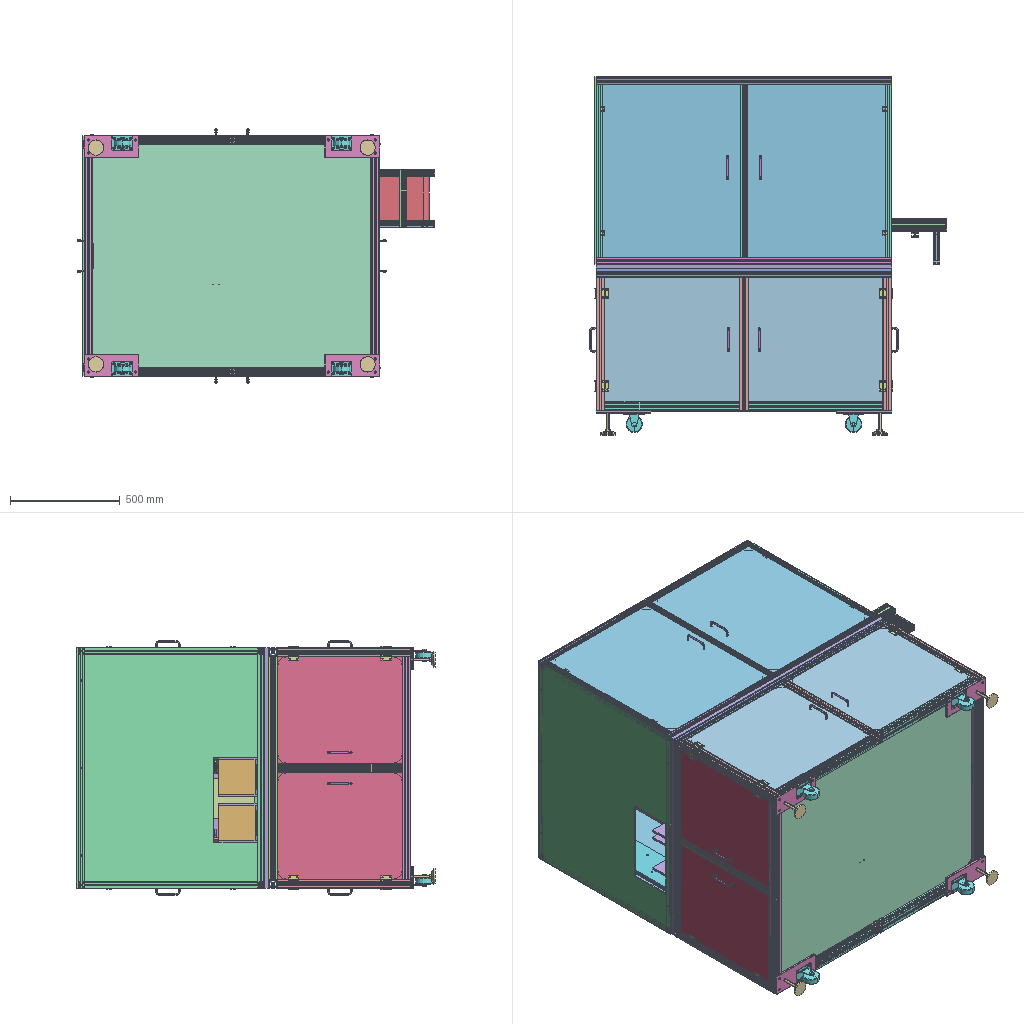Assembly | STEP file | 255 different items | 665 placed | box 1630 x 1635 x 1160 mm
Parts list (item | name | quantity | parent item | size | volume):
1 | 01-01 Bracket post | x6 | in 41 | 40 x 610 x 40 mm | 561060 mm3
2 | 01-03 Bracket crossbar 1 | x2 | in 41 | 40 x 1350 x 40 mm | 1241689 mm3
3 | 01-05 Bracket crossbar 3 | x2 | in 41 | 40 x 1020 x 40 mm | 938165 mm3
4 | 01-06 Bracket crossbar 4 | x2 | in 41 | 40 x 1020 x 40 mm | 938165 mm3
5 | 01-04 Bracket crossbar 2 | x4 | in 41 | 40 x 615 x 40 mm | 565659 mm3
6 | 01-02 Bracket post 2 | x2 | in 41 | 40 x 570 x 40 mm | 524269 mm3
7 | 01-07 Base plate | x1 | in 41 | 20 x 1100 x 1350 mm | 29158066 mm3
8 | 40×40 aluminium angle | x32 | in 41 | 30 x 40 x 40 mm | 8764 mm3
9 | 01-08 Base frame seal plate 1 | x4 | in 41 | 5 x 570 x 490 mm | 144415 mm3
10 | 01-09 Base frame seal plate 2 | x4 | in 41 | 5 x 570 x 615 mm | 180603 mm3
11 | 50 hinge | x16 | in 41 | 47 x 5 x 34 mm | 2311 mm3
12 | Stainless steel handle | x15 | in 41 | 8 x 30 x 112 mm | 7163 mm3
13 | 01-10 Base plate 2 | x1 | in 41 | 10 x 1330 x 1080 mm | 14031243 mm3
14 | 01-13 Coil feed support base plate | x1 | in 41 | 10 x 50 x 50 mm | 22250 mm3
15 | 01-12 Coil feed support plate | x1 | in 41 | 10 x 250 x 50 mm | 123839 mm3
16 | 01-11 Coil feed support shaft | x1 | in 41 | 50 x 40 x 40 mm | 62215 mm3
17 | 01-14 Caster foot cup support plate | x4 | in 41 | 10 x 250 x 100 mm | 245227 mm3
18 | Caster | x4 | in 41 | 70 x 95 x 87.5 mm | 164739 mm3
19 | Foot cup NFJNS16-130 | x4 | in 41 | 70 x 150 x 70 mm | 67181 mm3
20 | 05-01 Turntable | x1 | in 41 | 15 x 500 x 500 mm | 2906258 mm3
21 | 05-02 Turntable shaft | x1 | in 41 | 110 x 258 x 110 mm | 522826 mm3
22 | Bearing 32911 | x2 | in 41 | 80 x 17 x 80 mm | 44892 mm3
23 | 05-03 Turntable seat | x1 | in 41 | 150 x 128 x 150 mm | 603065 mm3
24 | 05-04 Turntable bottom press plate | x1 | in 41 | 10 x 70 x 70 mm | 31647 mm3
25 | 05-05 Fixture | x16 | in 41 | 42 x 40 x 40 mm | 49529 mm3
26 | Magnet dia 10 thickness 6 | x16 | in 41 | 6 x 10 x 10 mm | 467.969 mm3
27 | 05-06 Alignment piece fixing seat | x1 | in 41 | 45 x 45 x 20 mm | 12273 mm3
28 | 05-07 Alignment piece | x1 | in 41 | 2 x 69.821 x 69.821 mm | 5865 mm3
29 | Coupling CPSWWKΦ19-Φ19 (high-rigidity diaphragm type) | x1 | in 41 | 65 x 65 x 77 mm | 150728 mm3
30 | BSHB311 Baishan Motor | x1 | in 41 | 256 x 110 x 110 mm | 2048364 mm3
31 | 05-08 Motor fixing plate | x1 | in 41 | 10 x 160 x 160 mm | 243023 mm3
32 | 05-09 Fixing connection plate 1 | x4 | in 41 | 10 x 149 x 40 mm | 57725 mm3
33 | 05-10 Fixing connection plate 2 | x4 | in 41 | 10 x 149 x 30 mm | 43468 mm3
34 | 06-01 Heat-shrink sleeve shaft | x1 | in 41 | 20.3 x 500 x 20.3 mm | 156269 mm3
35 | Bearing B603ZZ | x4 | in 41 | 5 x 9 x 9 mm | 282.092 mm3
36 | 06-04 Bearing pin | x4 | in 41 | 12 x 3 x 3 mm | 82.729 mm3
37 | 06-02 Support feed wheel | x2 | in 41 | 20 x 25.8 x 25.8 mm | 8769 mm3
38 | 06-05 Support feed wheel shaft | x2 | in 41 | 12 x 12 x 67 mm | 4710 mm3
39 | Bearing B6900ZZ | x2 | in 41 | 6 x 22 x 22 mm | 1808 mm3
40 | circlips for shaft--type a large gb_GB_CONNECTING_PIECE_RING_RRA 10 | x2 | in 41 | 11.5 x 13.997 x 1 mm | 50.603 mm3
41 | 06-06 Driving feed support plate | x1 | in 41 | 10 x 260 x 100 mm | 216439 mm3
42 | 06-07 Bearing cover plate | x2 | in 41 | 2 x 60 x 30 mm | 2906 mm3
43 | hexagon socket head cap screws gb_GB_FASTENER_SCREWS_HSHCS M5X25-N | x4 | in 41 | 30 x 8.5 x 8.5 mm | 732.663 mm3
44 | BS57 Baishan Motor | x4 | in 41 | 98.2 x 56.4 x 56.4 mm | 213692 mm3
45 | 06-08 1-60 gear | x1 | in 41 | 20 x 61.958 x 61.958 mm | 30335 mm3
46 | 06-09 1-40 gear | x2 | in 41 | 20 x 41.938 x 41.938 mm | 14422 mm3
47 | 06-10 Guide mixing wheel support shaft | x4 | in 41 | 8 x 10 x 34 mm | 879.659 mm3
48 | Bearing B685ZZ | x8 | in 41 | 5 x 11 x 11 mm | 376.118 mm3
49 | 06-03 Guide mixing wheel | x4 | in 41 | 30 x 20 x 30 mm | 7202 mm3
50 | 06-11 Driven feed support plate | x1 | in 41 | 10 x 260 x 70 mm | 174356 mm3
51 | 06-12 Driving feed slide plate | x2 | in 41 | 25 x 80 x 70 mm | 132614 mm3
52 | 06-13 Push-pull bearing seat | x2 | in 41 | 16 x 30 x 45 mm | 7960 mm3
53 | Bearing B688ZZ | x2 | in 41 | 5 x 16 x 16 mm | 752.708 mm3
54 | 06-14 Bearing seat cover plate | x2 | in 41 | 5 x 25 x 25 mm | 2010 mm3
55 | 06-15 Slide guide block 1 | x4 | in 41 | 70 x 30 x 25 mm | 33661 mm3
56 | 06-16 M12 screw rod | x2 | in 41 | 12 x 12 x 75 mm | 7389 mm3
57 | Handwheel | x2 | in 41 | 80 x 80 x 65 mm | 48947 mm3
58 | 06-17 Screw locking block | x2 | in 41 | 15 x 60 x 45 mm | 23099 mm3
59 | 06-18 Fixing plate 1 | x1 | in 41 | 15 x 290 x 330 mm | 1410593 mm3
60 | 06-19 Stator fixing plate | x1 | in 41 | 10 x 140 x 140 mm | 144589 mm3
61 | 06-20 Stator core | x1 | in 41 | 81 x 55 x 55 mm | 107790 mm3
62 | 1/8 Φ8 fitting | x1 | in 41 | 28 x 16.166 x 14 mm | 2653 mm3
63 | Inner dia 42.5 wire dia 2.65 O-ring | x4 | in 41 | 47.7 x 47.7 x 2.6 mm | 752.251 mm3
64 | Bearing SB6909ZZ | x2 | in 41 | 12 x 68 x 68 mm | 24454 mm3
65 | 06-21 Rotor | x1 | in 41 | 147.929 x 147.929 x 62 mm | 569803 mm3
66 | 06-22 Stator support plate | x1 | in 41 | 10 x 50 x 50 mm | 13234 mm3
67 | 06-23 Rotor support plate | x1 | in 41 | 10 x 120 x 120 mm | 106201 mm3
68 | 06-25 Cutter slider | x1 | in 41 | 15 x 25 x 31 mm | 8782 mm3
69 | 06-27 Cutter cylinder fixing block | x1 | in 41 | 10 x 30 x 40 mm | 7335 mm3
70 | Cylinder CCOMPANY_AB 10-5_Retract | x1 | in 41 | 15 x 15 x 32.5 mm | 3211 mm3
71 | 06-24 Cutter slide rail | x2 | in 41 | 20 x 10 x 12 mm | 1659 mm3
72 | 06-26 Cutter press block | x1 | in 41 | 15 x 4 x 23 mm | 1168 mm3
73 | Insert blade | x1 | in 41 | 0.5 x 9 x 31.197 mm | 111.216 mm3
74 | 40W JSCC motor | x1 | in 41 | 143 x 125 x 90 mm | 815322 mm3
75 | 06-28 Gear 2-72 | x1 | in 41 | 50 x 147.929 x 147.929 mm | 253016 mm3
76 | 06-29 Up-down adjusting dovetail plate | x1 | in 41 | 230 x 20 x 150 mm | 590829 mm3
77 | 06-31 Dovetail fixing triangle plate | x4 | in 41 | 12 x 59.646 x 59.75 mm | 20836 mm3
78 | 06-32 Up-down adjusting dovetail groove | x1 | in 41 | 260 x 20 x 180 mm | 636123 mm3
79 | 06-30 Up-down dovetail press strip | x1 | in 41 | 260 x 10 x 12.002 mm | 13000 mm3
80 | 06-33 Front-rear adjusting dovetail plate | x1 | in 41 | 160 x 26 x 180 mm | 473686 mm3
81 | 06-34 Front-rear adjusting dovetail groove | x1 | in 41 | 140 x 26 x 110 mm | 222237 mm3
82 | 06-35 Front-rear dovetail press strip | x1 | in 41 | 140 x 16 x 16.203 mm | 11200 mm3
83 | 06-36 Front-rear dovetail base plate | x1 | in 41 | 10 x 140 x 240 mm | 326475 mm3
84 | 06-37 Heat-shrink tube support column | x4 | in 41 | 12 x 400 x 30 mm | 142471 mm3
85 | 06-38 Heat-shrink tube support crossbar | x2 | in 41 | 10 x 30 x 330 mm | 96911 mm3
86 | 06-39 Heat-shrink tube guide shaft | x3 | in 41 | 246 x 20 x 20 mm | 76812 mm3
87 | Inner dia 6 wire dia 1.8 O-ring | x1 | in 41 | 9.6 x 9.6 x 1.8 mm | 62.351 mm3
88 | 06-40 Flat key | x2 | in 41 | 3 x 3 x 13 mm | 111.206 mm3
89 | 40W JSCC gear motor | x1 | in 41 | 78 x 90 x 90 mm | 369652 mm3
90 | 02-04 Side frame | x1 | in 41 | 60 x 1495 x 30 mm | 1200559 mm3
91 | 02-03 Driving mixing drum support seat | x1 | in 41 | 60 x 60 x 30 mm | 91539 mm3
92 | Bearing 6802zz | x6 | in 41 | 5 x 24 x 24 mm | 1309 mm3
93 | 02-01 Driving mixing drum | x1 | in 41 | 50 x 50 x 271 mm | 629819 mm3
94 | 02-05 Driving mixing drum support seat 2 | x1 | in 41 | 60 x 60 x 30 mm | 91539 mm3
95 | 02-06 Side frame 2 | x1 | in 41 | 60 x 1495 x 30 mm | 1313620 mm3
96 | 02-07 25B driving sprocket | x1 | in 41 | 11 x 43.573 x 43.573 mm | 7127 mm3
97 | 02-08 Driving sprocket key | x1 | in 41 | 4 x 4 x 9.5 mm | 137.34 mm3
98 | 02-10 Motor fixing plate | x1 | in 41 | 30 x 130 x 100 mm | 33387 mm3
99 | Motor JSCC 25W | x1 | in 41 | 208 x 115 x 80 mm | 1081551 mm3
100 | 02-09 Motor sprocket | x1 | in 41 | 14 x 43.574 x 43.574 mm | 9063 mm3
101 | 25B chain | x1 | in 41 | 8.6 x 159.55 x 51.6 mm | 26237 mm3
102 | 02-11 Belt line support plate | x1 | in 41 | 1350 x 22 x 204 mm | 495672 mm3
103 | 02-12 Tensioning block 1 | x1 | in 41 | 20 x 32 x 32 mm | 16333 mm3
104 | 02-13 Tensioning block 2 | x1 | in 41 | 20 x 32 x 32 mm | 13018 mm3
105 | 02-02 Driven mixing drum | x1 | in 41 | 50 x 50 x 214 mm | 578580 mm3
106 | 02-14 Adjusting plate | x2 | in 41 | 5 x 60 x 30 mm | 8368 mm3
107 | 02-15 Belt line connecting rod | x4 | in 41 | 30 x 264 x 30 mm | 111601 mm3
108 | 02-15 Conveyor belt | x1 | in 41 | 200 x 54 x 1534 mm | 1249345 mm3
109 | 02-16 Belt line support foot | x8 | in 41 | 30 x 150 x 30 mm | 64799 mm3
110 | TN-16×125-S Extend | x1 | in 41 | 21 x 318 x 54 mm | 212013 mm3
111 | 02-17 Pusher cylinder fixing plate | x1 | in 41 | 10 x 264 x 120 mm | 277247 mm3
112 | Φ8 guide shaft seat | x4 | in 41 | 14 x 32.8 x 42 mm | 8820 mm3
113 | 02-18 Pull-off block | x1 | in 41 | 10 x 14 x 45 mm | 4364 mm3
114 | 02-19 Separating mechanism seal plate | x1 | in 41 | 15 x 350 x 264 mm | 1110870 mm3
115 | 02-20 Φ8 polished rod | x2 | in 41 | 244 x 8 x 8 mm | 12259 mm3
116 | Cylinder TN-16-10-S Retract | x1 | in 41 | 21 x 78 x 54 mm | 81436 mm3
117 | 02-21 Push plate | x1 | in 41 | 15 x 120 x 171.5 mm | 143256 mm3
118 | 02-22 Push connecting block | x1 | in 41 | 15 x 35 x 112 mm | 46704 mm3
119 | Linear bearing LMU8 | x6 | in 41 | 24 x 15 x 15 mm | 2999 mm3
120 | 02-23 Sprocket cover | x1 | in 41 | 40 x 180 x 80 mm | 22772 mm3
121 | 02-24 Battery support plate | x1 | in 41 | 120 x 60 x 120.818 mm | 18521 mm3
122 | Linear bearing LHFRD 16 | x4 | in 41 | 48 x 48 x 56 mm | 29540 mm3
123 | Lead screw head | x3 | in 41 | 44 x 50 x 34 mm | 38804 mm3
124 | 03-01 Loading-unloading side plate 1 | x2 | in 41 | 10 x 210 x 180 mm | 373986 mm3
125 | 03-02 Loading-unloading side plate 2 | x4 | in 41 | 10 x 210 x 168 mm | 351568 mm3
126 | 300 Lead screw | x2 | in 41 | 15 x 15 x 300 mm | 45152 mm3
127 | Bearing SB6800ZZ | x2 | in 41 | 5 x 19 x 19 mm | 1023 mm3
128 | 03-03 Tray support plate | x2 | in 41 | 15 x 168 x 160 mm | 317269 mm3
129 | Coupling CPJC 20 RD φ6.35-φ8 | x2 | in 41 | 30 x 20 x 20 mm | 7655 mm3
130 | 03-04 Bearing cover plate | x2 | in 41 | 5 x 36 x 36 mm | 3710 mm3
131 | 03-05 Motor fixing plate | x2 | in 41 | 8 x 70 x 140 mm | 77118 mm3
132 | 03-06 φ16 polished rod | x4 | in 41 | 320 x 16 x 16 mm | 64078 mm3
133 | 03-10 Bearing cover plate 2 | x2 | in 41 | 2 x 12 x 12 mm | 192.313 mm3
134 | 03-07 Feed mechanism support plate | x1 | in 41 | 10 x 609 x 168 mm | 1012240 mm3
135 | 03-08 Support plate base | x2 | in 41 | 70 x 10 x 168 mm | 114407 mm3
136 | 03-09 Support plate triangle plate | x4 | in 41 | 10 x 500 x 50 mm | 239136 mm3
137 | 03-11 Suction cup fixing plate | x1 | in 41 | 5 x 168 x 160 mm | 109255 mm3
138 | 03-12 Battery stop plate | x1 | in 41 | 15 x 168 x 160 mm | 313434 mm3
139 | Suction nozzle SRKN10+SRP9 | x4 | in 41 | 19.039 x 17.729 x 57.5 mm | 5768 mm3
140 | 03-13 Suction column | x25 | in 41 | 85 x 14 x 14 mm | 12701 mm3
141 | Magnet dia 8 thickness 3 | x25 | in 41 | 3 x 8 x 8 mm | 150.376 mm3
142 | 03-14 Suction column fixing plate | x1 | in 41 | 10 x 168 x 160 mm | 247896 mm3
143 | Cylinder CDQ2A-20×30-DM Extend | x1 | in 41 | 98 x 36 x 36 mm | 59217 mm3
144 | 03-15 Suction column cylinder fixing plate | x1 | in 41 | 10 x 168 x 160 mm | 252042 mm3
145 | Cylinder CDQ2A-32×20-DM Retract | x1 | in 41 | 86.5 x 45 x 45 mm | 118122 mm3
146 | 03-16 Φ8 column | x4 | in 41 | 153 x 8 x 8 mm | 7438 mm3
147 | Linear bearing LHMRD 10 | x4 | in 41 | 40 x 40 x 47 mm | 14628 mm3
148 | 03-17 Suction mechanism fixing plate | x1 | in 41 | 10 x 168 x 160 mm | 264041 mm3
149 | 03-18 Φ10 suction mechanism guide post | x4 | in 41 | 150 x 10 x 10 mm | 11525 mm3
150 | Linear bearing LHBB-MX 20 | x2 | in 41 | 64 x 41 x 54 mm | 104537 mm3
151 | 03-19 Lead screw head fixing plate 1 | x1 | in 41 | 10 x 50 x 50 mm | 14571 mm3
152 | 03-20 Lead screw head fixing plate 2 | x1 | in 41 | 30 x 10 x 50 mm | 14346 mm3
153 | 350 Lead screw | x1 | in 41 | 15 x 15 x 800 mm | 123903 mm3
154 | Bearing B6800ZZ | x2 | in 41 | 5 x 19 x 19 mm | 1023 mm3
155 | 03-21 Lead screw fixing plate | x1 | in 41 | 10 x 70 x 168 mm | 112553 mm3
156 | 03-22 Lead screw fixing plate rib | x4 | in 41 | 10 x 50 x 60 mm | 21700 mm3
157 | 03-23 Lead screw guide shaft | x2 | in 41 | 775 x 20 x 20 mm | 242804 mm3
158 | Coupling CPS-φ6.35-φ8 | x1 | in 41 | 25 x 25 x 25 mm | 9924 mm3
159 | 03-24 Feed mechanism support plate 2 | x1 | in 41 | 10 x 609 x 168 mm | 1013118 mm3
160 | 03-25 Support cross plate | x1 | in 41 | 10 x 168 x 835 mm | 1395635 mm3
161 | 04-02 Suction guide sleeve | x1 | in 41 | 40 x 60 x 40 mm | 20789 mm3
162 | 04-01 Φ12 chrome-plated rod | x1 | in 41 | 335 x 12 x 12 mm | 37192 mm3
163 | 04-03 Suction nozzle link | x1 | in 41 | 8 x 25 x 135 mm | 23811 mm3
164 | Suction nozzle SRKN10+SRP15 | x2 | in 41 | 19.039 x 17.729 x 57.5 mm | 6399 mm3
165 | 04-04 Suction gear | x1 | in 41 | 32 x 25 x 31.918 mm | 9255 mm3
166 | Bearing SB634ZZ | x1 | in 41 | 5 x 16 x 16 mm | 935.765 mm3
167 | circlips for holes--type a gb_GB_CONNECTING_PIECE_RING_RRH 16 | x1 | in 41 | 17.3 x 16.642 x 1 mm | 79.55 mm3
168 | Cylinder SDAJS 20×40-30 Retract | x1 | in 41 | 167.5 x 36 x 34 mm | 91234 mm3
169 | 04-05 Suction cylinder support rod | x4 | in 41 | 192 x 10 x 10 mm | 14822 mm3
170 | 04-06 Suction cylinder fixing plate | x1 | in 41 | 10 x 140 x 140 mm | 191449 mm3
171 | 04-08 Rack support plate | x1 | in 41 | 200 x 60 x 20 mm | 189566 mm3
172 | 04-07 Rotary feed rack | x1 | in 41 | 15 x 16 x 95 mm | 20700 mm3
173 | Cylinder MALJ 16×75-40-S Extend | x1 | in 41 | 351 x 22 x 22 mm | 68468 mm3
174 | 04-09 Suction rotary cylinder fixing plate | x1 | in 41 | 8 x 30 x 45 mm | 5704 mm3
175 | MHL2-10D_Open | x1 | in 41 | 46 x 44 x 100 mm | 98131 mm3
176 | 04-11 Guide cylinder raised bracket plate | x1 | in 41 | 10 x 270 x 50 mm | 130915 mm3
177 | 04-10 Guide cylinder fixing plate | x1 | in 41 | 10 x 90 x 50 mm | 42374 mm3
178 | 04-12 Guide cylinder base plate | x2 | in 41 | 50 x 10 x 50 mm | 22809 mm3
179 | 04-13 Guide block | x2 | in 41 | 12 x 26 x 34 mm | 8647 mm3
180 | 04-14 Guide reinforcing rib | x2 | in 41 | 10 x 130 x 35 mm | 41228 mm3
181 | Cylinder SDA S-12×10 Extend | x1 | in 41 | 52 x 25 x 25 mm | 21189 mm3
182 | 04-15 Heat-shrink tube press block | x1 | in 41 | 30 x 30 x 10 mm | 6743 mm3
183 | 04-16 Heat-shrink press cylinder fixing plate | x1 | in 41 | 10 x 90 x 50 mm | 43055 mm3
184 | 04-17 Heat-shrink press cylinder raised bracket plate | x1 | in 41 | 10 x 292 x 50 mm | 141915 mm3
185 | 03-26 Tray support slide plate | x2 | in 41 | 168 x 15 x 160 mm | 349859 mm3
186 | 08-01 Guard bracket 1 | x2 | in 41 | 30 x 1040 x 30 mm | 438839 mm3
187 | 08-02 Guard bracket 2 | x2 | in 41 | 30 x 1350 x 30 mm | 569484 mm3
188 | 08-03 Guard bracket 3 | x6 | in 41 | 30 x 790 x 30 mm | 333958 mm3
189 | 08-04 Guard bracket 4 | x2 | in 41 | 30 x 1040 x 30 mm | 439641 mm3
190 | 08-05 Guard bracket 5 | x2 | in 41 | 30 x 1350 x 30 mm | 570688 mm3
191 | 30×30 aluminium angle | x24 | in 41 | 20 x 36.5 x 36.5 mm | 8979 mm3
192 | 08-06 Guard top cover plate | x1 | in 41 | 5 x 1100 x 1350 mm | 7422677 mm3
193 | 08-07 Guard maintenance door | x4 | in 41 | 5 x 790 x 630 mm | 2488341 mm3
194 | 25 hinge-1 | x8 | in 41 | 25 x 4 x 12.7 mm | 342.439 mm3
195 | 25 hinge-2 | x8 | in 41 | 25 x 4 x 12.7 mm | 462.157 mm3
196 | 08-08 Seal plate | x1 | in 41 | 5 x 855 x 1100 mm | 4310509 mm3
197 | High-temperature rubber particle | x4 | in 41 | 15 x 21 x 10 mm | 685.576 mm3
198 | High-temperature rubber spring | x4 | in 41 | 8.7 x 6.5 x 6.5 mm | 27.892 mm3
199 | High-temperature rubber spring guide shaft | x4 | in 41 | 7.5 x 7.5 x 11 mm | 115.846 mm3
200 | 04-19 Up-down slide plate | x1 | in 41 | 10 x 160 x 160 mm | 241978 mm3
201 | Linear bearing LHFC 10 | x4 | in 41 | 29 x 40 x 25 mm | 9403 mm3
202 | 04-18 Gear support column | x1 | in 41 | 28 x 28 x 40 mm | 3984 mm3
203 | 09-37 Support plate base | x4 | in 41 | 10 x 50 x 60 mm | 26116 mm3
204 | 09-35 Support plate | x4 | in 41 | 10 x 315 x 60 mm | 183442 mm3
205 | 09-36 Support plate reinforcement plate | x4 | in 41 | 10 x 300 x 50 mm | 133768 mm3
206 | 09-34 Linear bearing shim | x8 | in 41 | 3 x 50 x 54 mm | 7702 mm3
207 | 09-02 Inner base plate 1 | x1 | in 41 | 1 x 350 x 425 mm | 63574 mm3
208 | 09-03 Inner base plate 2 | x1 | in 41 | 1 x 220 x 295 mm | 56061 mm3
209 | 09-04 Inner side plate 1 | x1 | in 41 | 410 x 172 x 35 mm | 76827 mm3
210 | 09-05 Inner side plate 2 | x1 | in 41 | 485 x 172 x 35 mm | 94551 mm3
211 | 09-06 Inner side plate 3 | x1 | in 41 | 410 x 172 x 35 mm | 73059 mm3
212 | 09-07 Inner side plate 4 | x1 | in 41 | 485 x 172 x 35 mm | 89624 mm3
213 | 09-08 Outer side plate 1 | x1 | in 41 | 5 x 195 x 410 mm | 399701 mm3
214 | 09-09 Outer side plate 2 | x1 | in 41 | 5 x 195 x 495 mm | 480012 mm3
215 | 09-10 Outer side plate 3 | x1 | in 41 | 5 x 195 x 410 mm | 380058 mm3
216 | 09-11 Outer side plate 4 | x1 | in 41 | 5 x 195 x 495 mm | 465621 mm3
217 | 09-12 Outer base plate 1 | x1 | in 41 | 5 x 420 x 495 mm | 502595 mm3
218 | 09-13 Outer base plate 2 | x1 | in 41 | 5 x 255 x 330 mm | 367508 mm3
219 | 09-14 Track outer side plate | x1 | in 41 | 48 x 281 x 356 mm | 23365 mm3
220 | 09-15 Track inner side plate | x1 | in 41 | 48 x 220 x 295 mm | 18723 mm3
221 | 09-16 Track outer seal plate | x1 | in 41 | 357 x 24 x 282 mm | 12816 mm3
222 | 09-17 Track inner end plate | x1 | in 41 | 24 x 221 x 296 mm | 10591 mm3
223 | 09-18 Outlet side seal plate 1 | x1 | in 41 | 73 x 1 x 33 mm | 2409 mm3
224 | 09-19 Outlet side seal plate 2 | x1 | in 41 | 73 x 1 x 38 mm | 2774 mm3
225 | 09-20 Outlet upper seal plate | x1 | in 41 | 1 x 29 x 94.448 mm | 2126 mm3
226 | 09-21 Inlet side seal plate | x1 | in 41 | 73 x 1 x 30 mm | 2190 mm3
227 | 09-22 Inlet side seal plate 2 | x1 | in 41 | 73 x 1 x 29.5 mm | 2153 mm3
228 | 09-23 Inlet upper seal plate | x1 | in 41 | 1 x 29 x 68.181 mm | 1787 mm3
229 | 09-24 Track cover plate | x1 | in 41 | 24 x 319 x 356 mm | 66305 mm3
230 | 09-25 Cover side plate 1 | x1 | in 41 | 35 x 5 x 420 mm | 72576 mm3
231 | 09-26 Cover side plate 2 | x1 | in 41 | 35 x 5 x 495 mm | 85750 mm3
232 | 09-27 Cover side plate 3 | x1 | in 41 | 35 x 5 x 420 mm | 72576 mm3
233 | 09-28 Cover side plate 4 | x1 | in 41 | 35 x 5 x 495 mm | 85493 mm3
234 | 09-29 Cover lid plate | x1 | in 41 | 34 x 410 x 485 mm | 320588 mm3
235 | 09-30 Cover base plate | x1 | in 41 | 4 x 410 x 485 mm | 203404 mm3
236 | Gas spring seat GSBR6B | x2 | in 41 | 40 x 34.1 x 40 mm | 7142 mm3
237 | Gas spring seat GSBR6C | x2 | in 41 | 40 x 34.1 x 40 mm | 7110 mm3
238 | Gas spring FGS 15089-100 rod | x2 | in 41 | 153 x 10 x 8.5 mm | 5670 mm3
239 | Gas spring FGS 15089-100 body | x2 | in 41 | 151 x 15 x 15 mm | 18389 mm3
240 | 70 hinge-1 | x2 | in 41 | 25.75 x 5.5 x 70 mm | 2438 mm3
241 | 70 hinge-2 | x2 | in 41 | 70 x 5.5 x 25.75 mm | 1924 mm3
242 | Guide shaft support SHAT-2025 | x8 | in 41 | 20 x 45 x 60 mm | 24589 mm3
243 | 09-31 Furnace lifting guide post | x4 | in 41 | 300 x 20 x 20 mm | 94187 mm3
244 | Bearing B6003ZZ | x1 | in 41 | 10 x 35 x 35 mm | 7334 mm3
245 | 09-32 Fan blade connecting shaft | x1 | in 41 | 20 x 20 x 76 mm | 14029 mm3
246 | 8-inch fan wheel | x1 | in 41 | 97 x 203 x 203 mm | 178976 mm3
247 | Coupling CPSφ12-φ12-φ25 | x1 | in 41 | 25 x 25 x 25 mm | 8428 mm3
248 | Motor TWT 5IK60A-C | x1 | in 41 | 191 x 90 x 90 mm | 1020211 mm3
249 | 09-33 Motor support plate | x2 | in 41 | 120 x 55 x 30 mm | 26486 mm3
250 | 09-39 Cylinder top plate | x1 | in 41 | 15 x 80 x 80 mm | 89624 mm3
251 | 09-01 Heating tube seat | x8 | in 41 | 10 x 25 x 13.5 mm | 303.936 mm3
252 | 09-40 Infeed pressure plate | x1 | in 41 | 18.5 x 120 x 59.46 mm | 10592 mm3
253 | Linear bearing LHBB-20 | x8 | in 41 | 50 x 41 x 54 mm | 78183 mm3
254 | 09-38 Cylinder pad plate | x1 | in 41 | 5 x 115 x 115 mm | 63470 mm3
255 | Cylinder SDA S-80×60 Retract | x1 | in 41 | 160 x 104 x 94 mm | 1037939 mm3
Placements (level | parent | child | x y z in mm | rotation matrix by rows), first 298 of 665 lines:
1 | 41 | 01-01 Bracket post | -784.116 3.376 -0.0 | 1 0 0 0 1 0 0 0 1
1 | 41 | 01-01 Bracket post | 525.884 3.376 -0.0 | 1 0 0 0 1 0 0 0 1
1 | 41 | 01-01 Bracket post | 525.884 3.376 -1060.0 | 1 0 0 0 1 0 0 0 1
1 | 41 | 01-01 Bracket post | -784.116 3.376 -1060.0 | 1 0 0 0 1 0 0 0 1
1 | 41 | 01-03 Bracket crossbar 1 | -129.116 328.376 -0.0 | 0 1 0 0 0 1 1 0 0
1 | 41 | 01-03 Bracket crossbar 1 | -129.116 328.376 -1060.0 | 0 -1 0 0 0 1 -1 0 0
1 | 41 | 01-05 Bracket crossbar 3 | -784.116 328.376 -530.0 | 0 0 -1 -1 0 0 0 1 0
1 | 41 | 01-05 Bracket crossbar 3 | 525.884 328.376 -530.0 | -1 0 0 0 0 1 0 1 0
1 | 41 | 01-06 Bracket crossbar 4 | 525.884 -281.624 -530.0 | 1 0 0 0 0 -1 0 1 0
1 | 41 | 01-06 Bracket crossbar 4 | -784.116 -281.624 -530.0 | 1 0 0 0 0 -1 0 1 0
1 | 41 | 01-04 Bracket crossbar 2 | 198.384 -281.624 -1060.0 | 0 1 0 -1 0 0 0 0 1
1 | 41 | 01-04 Bracket crossbar 2 | -456.616 -281.624 -1060.0 | 0 -1 0 1 0 0 0 0 1
1 | 41 | 01-04 Bracket crossbar 2 | -456.616 -281.624 -0.0 | 0 -1 0 1 0 0 0 0 1
1 | 41 | 01-04 Bracket crossbar 2 | 198.384 -281.624 -0.0 | 0 -1 0 1 0 0 0 0 1
1 | 41 | 01-02 Bracket post 2 | -784.116 23.376 -530.0 | 1 0 0 0 1 0 0 0 1
1 | 41 | 01-02 Bracket post 2 | 525.884 23.376 -530.0 | 1 0 0 0 1 0 0 0 1
1 | 41 | 01-07 Base plate | -129.116 348.376 -530.0 | 0 0 1 1 0 0 0 1 0
1 | 41 | 40×40 aluminium angle | -109.116 -261.624 -1060.0 | 0 0 -1 0 1 0 1 0 0
1 | 41 | 40×40 aluminium angle | 525.884 -261.624 -1040.0 | -1 0 0 0 1 0 0 0 -1
1 | 41 | 40×40 aluminium angle | -149.116 -261.624 -0.0 | 0 0 1 0 1 0 -1 0 0
1 | 41 | 40×40 aluminium angle | 505.884 -261.624 -0.0 | 0 0 1 0 1 0 -1 0 0
1 | 41 | 40×40 aluminium angle | -109.116 -261.624 -0.0 | 0 0 -1 0 1 0 1 0 0
1 | 41 | 40×40 aluminium angle | 525.884 -261.624 -510.0 | -1 0 0 0 1 0 0 0 -1
1 | 41 | 40×40 aluminium angle | 525.884 -261.624 -550.0 | 1 0 0 0 1 0 0 0 1
1 | 41 | 40×40 aluminium angle | 505.884 -261.624 -1060.0 | 0 0 1 0 1 0 -1 0 0
1 | 41 | 40×40 aluminium angle | -784.116 -261.624 -20.0 | 1 0 0 0 1 0 0 0 1
1 | 41 | 40×40 aluminium angle | -764.116 -261.624 -1060.0 | 0 0 -1 0 1 0 1 0 0
1 | 41 | 40×40 aluminium angle | -764.116 -261.624 -0.0 | 0 0 -1 0 1 0 1 0 0
1 | 41 | 40×40 aluminium angle | 525.884 -261.624 -20.0 | 1 0 0 0 1 0 0 0 1
1 | 41 | 40×40 aluminium angle | -149.116 -261.624 -1060.0 | 0 0 1 0 1 0 -1 0 0
1 | 41 | 40×40 aluminium angle | -784.116 -261.624 -1040.0 | -1 0 0 0 1 0 0 0 -1
1 | 41 | 40×40 aluminium angle | -784.116 308.376 -1040.0 | 1 0 0 0 -1 0 0 0 -1
1 | 41 | 40×40 aluminium angle | -784.116 308.376 -20.0 | 1 0 0 0 0 1 0 -1 0
1 | 41 | 40×40 aluminium angle | -109.116 308.376 -1060.0 | 0 1 0 0 0 1 1 0 0
1 | 41 | 40×40 aluminium angle | -784.116 308.376 -550.0 | 1 0 0 0 0 1 0 -1 0
1 | 41 | 40×40 aluminium angle | -149.116 308.376 0.0 | 0 -1 0 0 0 1 -1 0 0
1 | 41 | 40×40 aluminium angle | 505.884 308.376 -0.0 | 0 0 1 0 -1 0 1 0 0
1 | 41 | 40×40 aluminium angle | -109.116 308.376 0.0 | 0 0 -1 0 -1 0 -1 0 0
1 | 41 | 40×40 aluminium angle | -784.116 -261.624 -510.0 | -1 0 0 0 1 0 0 0 -1
1 | 41 | 40×40 aluminium angle | -784.116 -261.624 -550.0 | 1 0 0 0 1 0 0 0 1
1 | 41 | 40×40 aluminium angle | 525.884 308.376 -20.0 | 1 0 0 0 0 1 0 -1 0
1 | 41 | 40×40 aluminium angle | 525.884 308.376 -1040.0 | -1 0 0 0 0 1 0 1 0
1 | 41 | 40×40 aluminium angle | 525.884 308.376 -550.0 | 1 0 0 0 0 1 0 -1 0
1 | 41 | 40×40 aluminium angle | -764.116 308.376 -1060.0 | 0 1 0 0 0 1 1 0 0
1 | 41 | 40×40 aluminium angle | -784.116 308.376 -510.0 | -1 0 0 0 0 1 0 1 0
1 | 41 | 40×40 aluminium angle | -764.116 308.376 -0.0 | 0 1 0 0 0 1 1 0 0
1 | 41 | 40×40 aluminium angle | -149.116 308.376 -1060.0 | 0 0 1 0 -1 0 1 0 0
1 | 41 | 40×40 aluminium angle | 505.884 308.376 -1060.0 | 0 -1 0 0 0 1 -1 0 0
1 | 41 | 40×40 aluminium angle | 525.884 308.376 -510.0 | -1 0 0 0 0 1 0 1 0
1 | 41 | 01-08 Base frame seal plate 1 | 545.384 -261.624 -550.0 | 1 0 0 0 1 0 0 0 1
1 | 41 | 01-08 Base frame seal plate 1 | 545.384 -261.624 -20.0 | 1 0 0 0 1 0 0 0 1
1 | 41 | 01-08 Base frame seal plate 1 | -803.616 -261.624 -1040.0 | -1 0 0 0 1 0 0 0 -1
1 | 41 | 01-08 Base frame seal plate 1 | -803.616 -261.624 -510.0 | -1 0 0 0 1 0 0 0 -1
1 | 41 | 01-09 Base frame seal plate 2 | 505.884 -261.624 20.0 | 0 0 1 0 1 0 -1 0 0
1 | 41 | 01-09 Base frame seal plate 2 | -764.116 -261.624 -1080.0 | 0 0 -1 0 1 0 1 0 0
1 | 41 | 01-09 Base frame seal plate 2 | -109.116 -261.624 -1080.0 | 0 0 -1 0 1 0 1 0 0
1 | 41 | 01-09 Base frame seal plate 2 | -149.116 -261.624 20.0 | 0 0 1 0 1 0 -1 0 0
1 | 41 | 50 hinge | -804.116 234.876 -1040.0 | 0 1 0 -1 0 0 0 0 1
1 | 41 | 50 hinge | -804.116 -188.124 -1040.0 | 0 1 0 -1 0 0 0 0 1
1 | 41 | 50 hinge | -804.116 234.876 -20.0 | 0 1 0 -1 0 0 0 0 1
1 | 41 | 50 hinge | -764.116 234.876 20.0 | 0 0 1 -1 0 0 0 -1 0
1 | 41 | 50 hinge | -764.116 -188.124 20.0 | 0 0 1 -1 0 0 0 -1 0
1 | 41 | 50 hinge | -804.116 -188.124 -20.0 | 0 1 0 -1 0 0 0 0 1
1 | 41 | 50 hinge | 505.884 -188.124 20.0 | 0 0 -1 1 0 0 0 -1 0
1 | 41 | 50 hinge | 505.884 234.876 20.0 | 0 0 -1 1 0 0 0 -1 0
1 | 41 | 50 hinge | 545.884 234.876 -20.0 | 0 -1 0 1 0 0 0 0 1
1 | 41 | 50 hinge | 545.884 -188.124 -20.0 | 0 -1 0 1 0 0 0 0 1
1 | 41 | 50 hinge | 545.884 234.876 -1040.0 | 0 -1 0 1 0 0 0 0 1
1 | 41 | 50 hinge | 545.884 -188.124 -1040.0 | 0 -1 0 1 0 0 0 0 1
1 | 41 | 50 hinge | 505.884 234.876 -1080.0 | 0 0 -1 -1 0 0 0 1 0
1 | 41 | 50 hinge | -764.116 234.876 -1080.0 | 0 0 1 1 0 0 0 1 0
1 | 41 | 50 hinge | 505.884 -188.124 -1080.0 | 0 0 -1 -1 0 0 0 1 0
1 | 41 | 50 hinge | -764.116 -188.124 -1080.0 | 0 0 1 1 0 0 0 1 0
1 | 41 | Stainless steel handle | -59.116 23.376 -1080.0 | 1 0 0 0 0 -1 0 1 0
1 | 41 | Stainless steel handle | -199.116 23.376 -1080.0 | 1 0 0 0 0 -1 0 1 0
1 | 41 | Stainless steel handle | 545.884 23.376 -600.0 | 0 -1 0 0 0 1 -1 0 0
1 | 41 | Stainless steel handle | 545.884 23.376 -460.0 | 0 -1 0 0 0 -1 1 0 0
1 | 41 | Stainless steel handle | -59.116 23.376 20.0 | 1 0 0 0 0 1 0 -1 0
1 | 41 | Stainless steel handle | -199.116 23.376 20.0 | 1 0 0 0 0 1 0 -1 0
1 | 41 | Stainless steel handle | -804.116 23.376 -460.0 | 0 1 0 0 0 1 1 0 0
1 | 41 | Stainless steel handle | -804.116 23.376 -600.0 | 0 1 0 0 0 -1 -1 0 0
1 | 41 | 01-01 Bracket post | -129.116 3.376 -1060.0 | 1 0 0 0 1 0 0 0 1
1 | 41 | 01-01 Bracket post | -129.116 3.376 -0.0 | 1 0 0 0 1 0 0 0 1
1 | 41 | 01-10 Base plate 2 | -129.116 -261.624 -530.0 | 0 -1 0 1 0 0 0 0 1
1 | 41 | 01-13 Coil feed support base plate | -201.616 -251.624 -633.0 | 0 0 -1 1 0 0 0 -1 0
1 | 41 | 01-12 Coil feed support plate | -201.616 -251.124 -623.0 | 0 0 1 0 1 0 -1 0 0
1 | 41 | 01-11 Coil feed support shaft | -201.616 -51.124 -633.0 | 0 0 1 0 1 0 -1 0 0
1 | 41 | 01-14 Caster foot cup support plate | 545.884 -301.624 20.0 | 0 -1 0 -1 0 0 0 0 -1
1 | 41 | 01-14 Caster foot cup support plate | 545.884 -311.624 -1080.0 | 0 -1 0 1 0 0 0 0 1
1 | 41 | 01-14 Caster foot cup support plate | -804.116 -311.624 20.0 | 0 1 0 1 0 0 0 0 -1
1 | 41 | 01-14 Caster foot cup support plate | -804.116 -301.624 -1080.0 | 0 1 0 -1 0 0 0 0 1
1 | 41 | Caster | -629.616 -361.624 -15.0 | 0 1 0 0 0 1 1 0 0
1 | 41 | Caster | -629.616 -361.624 -1045.0 | 0 1 0 0 0 1 1 0 0
1 | 41 | Caster | 371.384 -361.624 -1045.0 | 0 -1 0 0 0 1 -1 0 0
1 | 41 | Caster | 371.384 -361.624 -15.0 | 0 -1 0 0 0 1 -1 0 0
1 | 41 | Foot cup NFJNS16-130 | -749.116 -401.658 -35.0 | 1 0 0 0 1 0 0 0 1
1 | 41 | Foot cup NFJNS16-130 | -749.116 -401.658 -1025.0 | 1 0 0 0 1 0 0 0 1
1 | 41 | Foot cup NFJNS16-130 | 490.884 -401.658 -35.0 | 1 0 0 0 1 0 0 0 1
1 | 41 | Foot cup NFJNS16-130 | 490.884 -401.658 -1025.0 | 1 0 0 0 1 0 0 0 1
1 | 41 | 05-01 Turntable | -14.116 521.376 -670.0 | 0 0 -1 1 0 0 0 -1 0
1 | 41 | 05-02 Turntable shaft | -14.116 521.376 -670.0 | 0.5 0 -0.866 0 1 0 0.866 0 0.5
1 | 41 | Bearing 32911 | -14.116 479.376 -670.0 | 0 0 -1 0 1 0 1 0 0
1 | 41 | 05-03 Turntable seat | -14.116 368.376 -670.0 | 0.5 0 0.866 0 1 0 -0.866 0 0.5
1 | 41 | Bearing 32911 | -14.116 368.376 -670.0 | 0 0 -1 0 1 0 1 0 0
1 | 41 | 05-04 Turntable bottom press plate | -14.116 358.376 -670.0 | 0 0 -1 1 0 0 0 -1 0
1 | 41 | 05-05 Fixture | -217.369 536.376 -754.19 | 0 0.3827 -0.9239 1 0 0 0 -0.9239 -0.3827
1 | 41 | 05-05 Fixture | 141.448 536.376 -825.563 | 0 0.7071 -0.7071 1 0 0 0 -0.7071 -0.7071
1 | 41 | 05-05 Fixture | 205.884 536.376 -670.0 | 0 1 0 1 0 0 0 0 -1
1 | 41 | 05-05 Fixture | 189.138 536.376 -585.81 | 0 0.3827 -0.9239 1 0 0 0 -0.9239 -0.3827
1 | 41 | 05-05 Fixture | 189.138 536.376 -754.19 | 0 0.3827 0.9239 1 0 0 0 0.9239 -0.3827
1 | 41 | 05-05 Fixture | -217.369 536.376 -585.81 | 0 -0.3827 -0.9239 1 0 0 0 -0.9239 0.3827
1 | 41 | 05-05 Fixture | -98.306 536.376 -873.254 | 0 -0.3827 -0.9239 1 0 0 0 -0.9239 0.3827
1 | 41 | 05-05 Fixture | 70.075 536.376 -873.254 | 0 0.3827 -0.9239 1 0 0 0 -0.9239 -0.3827
1 | 41 | 05-05 Fixture | -234.116 536.376 -670.0 | 0 0 -1 1 0 0 0 -1 0
1 | 41 | 05-05 Fixture | -169.679 536.376 -825.563 | 0 0.7071 -0.7071 1 0 0 0 -0.7071 -0.7071
1 | 41 | 05-05 Fixture | -14.116 536.376 -890.0 | 0 0 -1 1 0 0 0 -1 0
1 | 41 | 05-05 Fixture | -98.306 536.376 -466.747 | 0 0.3827 -0.9239 1 0 0 0 -0.9239 -0.3827
1 | 41 | 05-05 Fixture | -14.116 536.376 -450.0 | 0 0 -1 1 0 0 0 -1 0
1 | 41 | 05-05 Fixture | 141.448 536.376 -514.437 | 0 0.7071 -0.7071 1 0 0 0 -0.7071 -0.7071
1 | 41 | 05-05 Fixture | 70.075 536.376 -466.747 | 0 -0.3827 -0.9239 1 0 0 0 -0.9239 0.3827
1 | 41 | 05-05 Fixture | -169.679 536.376 -514.437 | 0 0.7071 -0.7071 1 0 0 0 -0.7071 -0.7071
1 | 41 | Magnet dia 10 thickness 6 | -217.369 571.376 -585.81 | 0 0 -1 1 0 0 0 -1 0
1 | 41 | Magnet dia 10 thickness 6 | 189.138 571.376 -754.19 | 0 0 -1 1 0 0 0 -1 0
1 | 41 | Magnet dia 10 thickness 6 | -14.116 571.376 -890.0 | 0 0 -1 1 0 0 0 -1 0
1 | 41 | Magnet dia 10 thickness 6 | 205.884 571.376 -670.0 | 0 0 -1 1 0 0 0 -1 0
1 | 41 | Magnet dia 10 thickness 6 | -169.679 571.376 -825.563 | 0 0 -1 1 0 0 0 -1 0
1 | 41 | Magnet dia 10 thickness 6 | -98.306 571.376 -466.747 | 0 0 -1 1 0 0 0 -1 0
1 | 41 | Magnet dia 10 thickness 6 | 141.448 571.376 -514.437 | 0 0 -1 1 0 0 0 -1 0
1 | 41 | Magnet dia 10 thickness 6 | -98.306 571.376 -873.254 | 0 0 -1 1 0 0 0 -1 0
1 | 41 | Magnet dia 10 thickness 6 | -234.116 571.376 -670.0 | 0 0 -1 1 0 0 0 -1 0
1 | 41 | Magnet dia 10 thickness 6 | -217.369 571.376 -754.19 | 0 0 -1 1 0 0 0 -1 0
1 | 41 | Magnet dia 10 thickness 6 | -169.679 571.376 -514.437 | 0 0 -1 1 0 0 0 -1 0
1 | 41 | Magnet dia 10 thickness 6 | -14.116 571.376 -450.0 | 0 0 -1 1 0 0 0 -1 0
1 | 41 | Magnet dia 10 thickness 6 | 70.075 571.376 -466.747 | 0 0 -1 1 0 0 0 -1 0
1 | 41 | Magnet dia 10 thickness 6 | 189.138 571.376 -585.81 | 0 0 -1 1 0 0 0 -1 0
1 | 41 | Magnet dia 10 thickness 6 | 70.075 571.376 -873.254 | 0 0 -1 1 0 0 0 -1 0
1 | 41 | Magnet dia 10 thickness 6 | 141.448 571.376 -825.563 | 0 0 -1 1 0 0 0 -1 0
1 | 41 | 05-06 Alignment piece fixing seat | -14.116 318.376 -670.0 | 0.5 0.866 0 0 0 1 0.866 -0.5 0
1 | 41 | 05-07 Alignment piece | -14.116 316.376 -670.0 | 0 0.866 -0.5 1 0 0 0 -0.5 -0.866
1 | 41 | Coupling CPSWWKΦ19-Φ19 (high-rigidity diaphragm type) | -14.116 283.376 -670.0 | -0.5 -0.866 0 0 0 1 -0.866 0.5 0
1 | 41 | BSHB311 Baishan Motor | -14.116 186.376 -670.0 | 0 1 0 -1 0 0 0 0 1
1 | 41 | 05-08 Motor fixing plate | -14.116 189.376 -670.0 | 0 0 -1 1 0 0 0 -1 0
1 | 41 | 05-09 Fixing connection plate 1 | -94.116 199.376 -590.0 | 1 0 0 0 1 0 0 0 1
1 | 41 | 05-09 Fixing connection plate 1 | 65.884 199.376 -590.0 | 0 0 1 0 1 0 -1 0 0
1 | 41 | 05-09 Fixing connection plate 1 | 65.884 199.376 -750.0 | -1 0 0 0 1 0 0 0 -1
1 | 41 | 05-09 Fixing connection plate 1 | -94.116 199.376 -750.0 | 0 0 -1 0 1 0 1 0 0
1 | 41 | 05-10 Fixing connection plate 2 | -94.116 348.376 -740.0 | 1 0 0 0 -1 0 0 0 -1
1 | 41 | 05-10 Fixing connection plate 2 | -84.116 348.376 -590.0 | 0 0 -1 0 -1 0 -1 0 0
1 | 41 | 05-10 Fixing connection plate 2 | 55.884 199.376 -600.0 | 1 0 0 0 1 0 0 0 1
1 | 41 | 05-10 Fixing connection plate 2 | 55.884 348.376 -750.0 | 0 0 1 0 -1 0 1 0 0
1 | 41 | 06-01 Heat-shrink sleeve shaft | -234.116 582.376 -670.0 | 0 0 -1 0 1 0 1 0 0
1 | 41 | Bearing B603ZZ | -234.116 907.376 -675.75 | -1 0 0 0 1 0 0 0 -1
1 | 41 | Bearing B603ZZ | -234.116 887.376 -675.75 | -1 0 0 0 1 0 0 0 -1
1 | 41 | Bearing B603ZZ | -234.116 887.376 -664.25 | -1 0 0 0 1 0 0 0 -1
1 | 41 | Bearing B603ZZ | -234.116 907.376 -664.25 | -1 0 0 0 1 0 0 0 -1
1 | 41 | 06-04 Bearing pin | -234.116 907.376 -664.25 | 1 0 0 0 1 0 0 0 1
1 | 41 | 06-04 Bearing pin | -234.116 907.376 -675.75 | 1 0 0 0 1 0 0 0 1
1 | 41 | 06-04 Bearing pin | -234.116 887.376 -664.25 | 1 0 0 0 1 0 0 0 1
1 | 41 | 06-04 Bearing pin | -234.116 887.376 -675.75 | 1 0 0 0 1 0 0 0 1
1 | 41 | 06-02 Support feed wheel | -234.116 897.376 -689.989 | 1 0 0 0 0.9793 0.2024 0 -0.2024 0.9793
1 | 41 | 06-05 Support feed wheel shaft | -217.116 897.376 -689.989 | 0 0 1 -0.2024 0.9793 0 -0.9793 -0.2024 0
1 | 41 | Bearing B6900ZZ | -257.116 897.376 -689.989 | 1 0 0 0 1 0 0 0 1
1 | 41 | 06-02 Support feed wheel | -234.116 897.376 -650.011 | 1 0 0 0 1 0 0 0 1
1 | 41 | 06-05 Support feed wheel shaft | -217.116 897.376 -650.011 | 0 0 1 0 1 0 -1 0 0
1 | 41 | Bearing B6900ZZ | -257.116 897.376 -650.011 | 1 0 0 0 1 0 0 0 1
1 | 41 | circlips for shaft--type a large gb_GB_CONNECTING_PIECE_RING_RRA 10 | -261.116 897.027 -689.903 | 0 0 -1 -0.2399 -0.9708 0 -0.9708 0.2399 0
1 | 41 | circlips for shaft--type a large gb_GB_CONNECTING_PIECE_RING_RRA 10 | -261.116 897.1 -650.241 | 0 0 -1 0.641 -0.7676 0 -0.7676 -0.641 0
1 | 41 | 06-06 Driving feed support plate | -252.116 897.376 -665.011 | -1 0 0 0 1 0 0 0 -1
1 | 41 | 06-07 Bearing cover plate | -260.116 897.376 -650.011 | -1 0 0 0 1 0 0 0 -1
1 | 41 | hexagon socket head cap screws gb_GB_FASTENER_SCREWS_HSHCS M5X25-N | -267.116 922.376 -640.011 | 1 0 0 0 -0.9237 -0.383 0 0.383 -0.9237
1 | 41 | hexagon socket head cap screws gb_GB_FASTENER_SCREWS_HSHCS M5X25-N | -267.116 922.376 -660.011 | 1 0 0 0 -0.9237 -0.383 0 0.383 -0.9237
1 | 41 | hexagon socket head cap screws gb_GB_FASTENER_SCREWS_HSHCS M5X25-N | -267.116 872.376 -640.011 | 1 0 0 0 -0.9237 -0.383 0 0.383 -0.9237
1 | 41 | hexagon socket head cap screws gb_GB_FASTENER_SCREWS_HSHCS M5X25-N | -267.116 872.376 -660.011 | 1 0 0 0 -0.9237 -0.383 0 0.383 -0.9237
1 | 41 | BS57 Baishan Motor | -257.116 897.376 -600.011 | 1 0 0 0 1 0 0 0 1
1 | 41 | 06-08 1-60 gear | -274.316 897.376 -600.011 | -1 0 0 0 0.9986 -0.05336 0 -0.05336 -0.9986
1 | 41 | 06-09 1-40 gear | -274.116 897.376 -650.011 | -1 0 0 0 -0.8896 0.4567 0 0.4567 0.8896
1 | 41 | 06-09 1-40 gear | -274.116 897.376 -689.989 | -1 0 0 0 -0.9237 0.383 0 0.383 0.9237
1 | 41 | 06-10 Guide mixing wheel support shaft | -218.116 997.376 -650.011 | 0 0 1 -1 0 0 0 -1 0
1 | 41 | 06-10 Guide mixing wheel support shaft | -218.116 797.376 -650.011 | 0 0 1 -1 0 0 0 -1 0
1 | 41 | Bearing B685ZZ | -241.616 997.376 -650.011 | 1 0 0 0 0.9386 0.345 0 -0.345 0.9386
1 | 41 | 06-03 Guide mixing wheel | -234.116 997.376 -650.011 | 0 -1 0 0.2134 0 -0.977 0.977 0 0.2134
1 | 41 | Bearing B685ZZ | -226.616 997.376 -650.011 | 1 0 0 0 1 0 0 0 1
1 | 41 | Bearing B685ZZ | -241.616 797.376 -650.011 | 1 0 0 0 1 0 0 0 1
1 | 41 | Bearing B685ZZ | -226.616 797.376 -650.011 | 1 0 0 0 1 0 0 0 1
1 | 41 | 06-03 Guide mixing wheel | -234.116 797.376 -650.011 | 0 1 0 0.000143 0 1 1 0 -0.000143
1 | 41 | 06-11 Driven feed support plate | -252.116 897.376 -674.989 | -1 0 0 0 1 0 0 0 -1
1 | 41 | 06-07 Bearing cover plate | -260.116 897.372 -689.989 | -1 0 0 0 1 0 0 0 -1
1 | 41 | 06-10 Guide mixing wheel support shaft | -218.116 997.376 -690.0 | 0 0 1 -1 0 0 0 -1 0
1 | 41 | 06-10 Guide mixing wheel support shaft | -218.116 797.376 -689.989 | 0 0 1 -1 0 0 0 -1 0
1 | 41 | Bearing B685ZZ | -241.616 997.376 -690.0 | 1 0 0 0 1 0 0 0 1
1 | 41 | Bearing B685ZZ | -226.616 797.376 -689.989 | 1 0 0 0 1 0 0 0 1
1 | 41 | Bearing B685ZZ | -226.616 997.376 -690.0 | 1 0 0 0 1 0 0 0 1
1 | 41 | Bearing B685ZZ | -241.616 797.376 -689.989 | 1 0 0 0 1 0 0 0 1
1 | 41 | 06-03 Guide mixing wheel | -234.116 997.376 -690.0 | 0 -1 0 -0.008522 0 -1 1 0 -0.008522
1 | 41 | 06-03 Guide mixing wheel | -234.116 797.376 -689.989 | 0 -1 0 -0.02818 0 -0.9996 0.9996 0 -0.02818
1 | 41 | 06-12 Driving feed slide plate | -257.116 742.376 -605.011 | 0 0 -1 1 0 0 0 -1 0
1 | 41 | 06-12 Driving feed slide plate | -257.116 742.376 -734.989 | 0 0 1 1 0 0 0 1 0
1 | 41 | 06-13 Push-pull bearing seat | -257.116 767.376 -581.011 | 0 0 -1 0 1 0 1 0 0
1 | 41 | Bearing B688ZZ | -257.116 784.876 -575.011 | 0 0 -1 0 1 0 1 0 0
1 | 41 | 06-14 Bearing seat cover plate | -257.116 784.876 -565.011 | 0 1 0 0 0 -1 -1 0 0
1 | 41 | 06-13 Push-pull bearing seat | -257.116 767.376 -758.989 | 0 0 1 0 1 0 -1 0 0
1 | 41 | Bearing B688ZZ | -257.116 784.876 -769.989 | 0 0 -1 0 1 0 1 0 0
1 | 41 | 06-14 Bearing seat cover plate | -257.116 784.876 -774.989 | 0 0 -1 0 1 0 1 0 0
1 | 41 | 06-15 Slide guide block 1 | -307.116 772.376 -600.011 | 0 0 -1 0 1 0 1 0 0
1 | 41 | 06-15 Slide guide block 1 | -207.116 772.376 -600.011 | 0 0 1 0 1 0 -1 0 0
1 | 41 | 06-15 Slide guide block 1 | -207.116 772.376 -739.989 | 0 0 1 0 1 0 -1 0 0
1 | 41 | 06-15 Slide guide block 1 | -307.116 772.376 -739.989 | 0 0 -1 0 1 0 1 0 0
1 | 41 | 06-16 M12 screw rod | -257.116 784.876 -578.811 | -1 0 0 0 1 0 0 0 -1
1 | 41 | Handwheel | -257.116 784.876 -493.811 | -1 0 0 0 1 0 0 0 -1
1 | 41 | 06-16 M12 screw rod | -257.116 784.876 -761.189 | 1 0 0 0 1 0 0 0 1
1 | 41 | Handwheel | -257.116 784.876 -846.189 | 1 0 0 0 1 0 0 0 1
1 | 41 | 06-17 Screw locking block | -257.116 742.376 -807.489 | 0 0 -1 0 1 0 1 0 0
1 | 41 | 06-17 Screw locking block | -257.116 742.376 -532.511 | 0 0 -1 0 1 0 1 0 0
1 | 41 | 06-18 Fixing plate 1 | -184.116 742.376 -670.0 | 0 0 -1 -1 0 0 0 1 0
1 | 41 | 06-19 Stator fixing plate | -234.116 717.376 -670.0 | 0 0.7071 -0.7071 1 0 0 0 -0.7071 -0.7071
1 | 41 | 06-20 Stator core | -234.116 717.376 -670.0 | 0 -1 0 -1 0 0 0 0 -1
1 | 41 | 1/8 Φ8 fitting | -268.616 702.376 -670.0 | -1 0 0 0 0.5869 0.8097 0 0.8097 -0.5869
1 | 41 | Inner dia 42.5 wire dia 2.65 O-ring | -234.32 672.026 -670.144 | 0 1 0 0 0 1 1 0 0
1 | 41 | Inner dia 42.5 wire dia 2.65 O-ring | -234.149 668.326 -670.248 | 0 1 0 0 0 1 1 0 0
1 | 41 | Inner dia 42.5 wire dia 2.65 O-ring | -233.869 655.426 -670.043 | 0 1 0 0 0 1 1 0 0
1 | 41 | Inner dia 42.5 wire dia 2.65 O-ring | -233.886 651.726 -670.099 | 0 1 0 0 0 1 1 0 0
1 | 41 | Bearing SB6909ZZ | -234.116 681.376 -670.0 | 0 0 -1 1 0 0 0 -1 0
1 | 41 | Bearing SB6909ZZ | -234.116 642.376 -670.0 | 0 0 -1 1 0 0 0 -1 0
1 | 41 | 06-21 Rotor | -234.116 687.376 -670.0 | 0.9922 0.1246 0 0 0 1 0.1246 -0.9922 0
1 | 41 | 06-22 Stator support plate | -234.116 636.376 -670.0 | 0 -0.7071 0.7071 -1 0 0 0 -0.7071 -0.7071
1 | 41 | 06-23 Rotor support plate | -234.116 625.376 -670.0 | 0 0.6135 -0.7897 -1 0 0 0 0.7897 0.6135
1 | 41 | 06-25 Cutter slider | -235.121 615.376 -625.881 | 0.1246 0 -0.9922 0 -1 0 -0.9922 0 -0.1246
1 | 41 | 06-27 Cutter cylinder fixing block | -236.616 615.376 -613.975 | 0.1246 0 -0.9922 0 -1 0 -0.9922 0 -0.1246
1 | 41 | Cylinder CCOMPANY_AB 10-5_Retract | -235.37 597.376 -623.897 | -0.9922 0 0.1246 0 1 0 -0.1246 0 -0.9922
1 | 41 | 06-24 Cutter slide rail | -210.571 615.376 -632.776 | -0.1246 0 0.9922 0 -1 0 0.9922 0 0.1246
1 | 41 | 06-26 Cutter press block | -234.186 586.876 -633.323 | -0.1246 0 -0.9922 0 1 0 0.9922 0 -0.1246
1 | 41 | 06-24 Cutter slide rail | -257.204 615.376 -638.633 | 0.1246 0 -0.9922 0 -1 0 -0.9922 0 -0.1246
1 | 41 | Insert blade | -230.905 590.126 -623.336 | 0 -0.9922 -0.1246 1 0 0 0 -0.1246 0.9922
1 | 41 | 40W JSCC motor | -360.116 788.376 -670.0 | 0 -1 0 1 0 0 0 0 1
1 | 41 | 06-28 Gear 2-72 | -378.116 679.876 -670.0 | 0 0.6608 -0.7506 -1 0 0 0 0.7506 0.6608
1 | 41 | 06-29 Up-down adjusting dovetail plate | -464.116 612.376 -670.0 | 0 -1 0 1 0 0 0 0 1
1 | 41 | 06-31 Dovetail fixing triangle plate | -454.116 727.376 -601.0 | 0 1 0 0 0 1 1 0 0
1 | 41 | 06-31 Dovetail fixing triangle plate | -454.116 727.376 -739.0 | 0 1 0 0 0 1 1 0 0
1 | 41 | 06-32 Up-down adjusting dovetail groove | -484.116 414.376 -670.0 | 0 -1 0 1 0 0 0 0 1
1 | 41 | 06-30 Up-down dovetail press strip | -474.116 674.376 -610.0 | 0 1 0 -1 0 0 0 0 1
1 | 41 | 06-31 Dovetail fixing triangle plate | -464.116 414.376 -586.0 | 0 0 -1 0 1 0 1 0 0
1 | 41 | 06-31 Dovetail fixing triangle plate | -464.116 414.376 -754.0 | 0 0 -1 0 1 0 1 0 0
1 | 41 | 06-33 Front-rear adjusting dovetail plate | -324.116 414.376 -670.0 | -1 0 0 0 1 0 0 0 -1
1 | 41 | 06-34 Front-rear adjusting dovetail groove | -464.116 378.376 -670.0 | 1 0 0 0 1 0 0 0 1
1 | 41 | 06-35 Front-rear dovetail press strip | -464.116 388.376 -625.0 | 1 0 0 0 1 0 0 0 1
1 | 41 | 06-36 Front-rear dovetail base plate | -394.116 368.376 -670.0 | 0 -1 0 1 0 0 0 0 1
1 | 41 | 06-37 Heat-shrink tube support column | -469.116 742.376 -803.0 | 0 0 1 0 1 0 -1 0 0
1 | 41 | 06-37 Heat-shrink tube support column | -469.116 742.376 -537.0 | 0 0 -1 0 1 0 1 0 0
1 | 41 | 06-37 Heat-shrink tube support column | -169.116 742.376 -803.0 | 0 0 1 0 1 0 -1 0 0
1 | 41 | 06-37 Heat-shrink tube support column | -169.116 742.376 -537.0 | 0 0 -1 0 1 0 1 0 0
1 | 41 | 06-38 Heat-shrink tube support crossbar | -319.116 1127.376 -793.0 | 0 0 1 0 1 0 -1 0 0
1 | 41 | 06-38 Heat-shrink tube support crossbar | -319.116 1127.376 -547.0 | 0 0 1 0 -1 0 1 0 0
1 | 41 | 06-39 Heat-shrink tube guide shaft | -223.116 1127.376 -670.0 | 0 0 -1 0 1 0 1 0 0
1 | 41 | 06-39 Heat-shrink tube guide shaft | -245.116 1127.376 -670.0 | 0 0 -1 0 1 0 1 0 0
1 | 41 | 06-39 Heat-shrink tube guide shaft | -447.116 1127.376 -670.0 | 0 0 -1 0 1 0 1 0 0
1 | 41 | Inner dia 6 wire dia 1.8 O-ring | -252.116 716.876 -670.0 | 0 1 0 0 0 1 1 0 0
1 | 41 | 06-40 Flat key | -239.116 903.448 -691.244 | 0 0 -1 -0.9793 0.2024 0 0.2024 0.9793 0
1 | 41 | 06-40 Flat key | -239.116 903.576 -650.011 | 0 0 -1 -1 0 0 0 1 0
1 | 41 | 40W JSCC gear motor | -360.116 788.376 -670.0 | 0 1 0 -1 0 0 0 0 1
1 | 41 | 02-04 Side frame | 43.384 548.376 -385.0 | 0 -1 0 -1 0 0 0 0 -1
1 | 41 | 02-03 Driving mixing drum support seat | -704.116 548.376 -385.0 | -1 0 0 0 1 0 0 0 -1
1 | 41 | Bearing 6802zz | -734.116 550.376 -377.5 | 0 -1 0 0 0 -1 1 0 0
1 | 41 | Bearing 6802zz | -734.116 550.376 -372.5 | 0 -1 0 0 0 -1 1 0 0
1 | 41 | 02-01 Driving mixing drum | -734.116 550.376 -427.0 | -0.9859 -0.1676 0 -0.1676 0.9859 0 0 0 -1
1 | 41 | Bearing 6802zz | -734.116 550.376 -163.5 | 0 -1 0 0 0 1 -1 0 0
1 | 41 | Bearing 6802zz | -734.116 550.376 -158.5 | 0 -1 0 0 0 1 -1 0 0
1 | 41 | 02-05 Driving mixing drum support seat 2 | -704.116 548.376 -151.0 | -1 0 0 0 -1 0 0 0 1
1 | 41 | 02-06 Side frame 2 | 43.384 548.376 -151.0 | 0 -1 0 -1 0 0 0 0 -1
1 | 41 | 02-07 25B driving sprocket | -734.116 550.376 -418.6 | 0 -0.1676 -0.9859 0 0.9859 -0.1676 1 0 0
1 | 41 | 02-08 Driving sprocket key | -735.373 557.77 -416.5 | 0.1676 -0.9859 0 -0.9859 -0.1676 0 0 0 -1
1 | 41 | 02-10 Motor fixing plate | -654.116 388.376 -400.0 | 0 0 1 0 1 0 -1 0 0
1 | 41 | Motor JSCC 25W | -654.116 463.376 -398.5 | 0 -1e-06 1 0 -1 -1e-06 1 0 0
1 | 41 | 02-09 Motor sprocket | -654.116 478.376 -420.0 | 0 -1e-06 1 0 -1 -1e-06 1 0 0
1 | 41 | 25B chain | -652.85 479.319 -422.0 | 0 -0.7528 -0.6582 0 0.6582 -0.7528 1 0 0
1 | 41 | 02-11 Belt line support plate | 665.884 553.376 -243.0 | -1 0 0 0 1 0 0 0 -1
1 | 41 | 02-12 Tensioning block 1 | 745.884 548.376 -390.0 | 0 0 -1 0 1 0 1 0 0
1 | 41 | 02-13 Tensioning block 2 | 745.884 548.376 -146.0 | 0 0 -1 0 -1 0 -1 0 0
1 | 41 | Bearing 6802zz | 745.884 550.376 -372.5 | 0 -1 0 0 0 -1 1 0 0
1 | 41 | Bearing 6802zz | 745.884 550.376 -163.5 | 0 -1 0 0 0 1 -1 0 0
1 | 41 | 02-02 Driven mixing drum | 745.884 550.376 -375.0 | 0.06134 -0.9981 0 -0.9981 -0.06134 0 0 0 -1
1 | 41 | 02-14 Adjusting plate | 795.884 548.376 -385.0 | -1 0 0 0 -1 0 0 0 1
1 | 41 | 02-14 Adjusting plate | 790.884 548.376 -151.0 | 1 0 0 0 -1 0 0 0 -1
1 | 41 | 02-15 Belt line connecting rod | -549.116 503.376 -268.0 | 0 0 -1 -1 0 0 0 1 0
1 | 41 | 02-15 Belt line connecting rod | -149.116 503.376 -268.0 | 0 0 1 -1 0 0 0 -1 0
1 | 41 | 02-15 Belt line connecting rod | 250.884 503.376 -268.0 | 0 0 1 -1 0 0 0 -1 0
1 | 41 | 02-15 Conveyor belt | 5.884 550.376 -268.0 | 0 0 1 0 1 0 -1 0 0
1 | 41 | 02-16 Belt line support foot | -49.116 443.376 -151.0 | -1 0 0 0 1 0 0 0 -1
1 | 41 | 02-16 Belt line support foot | 350.884 443.376 -385.0 | -1 0 0 0 1 0 0 0 -1
1 | 41 | 02-16 Belt line support foot | -49.116 443.376 -385.0 | -1 0 0 0 1 0 0 0 -1
1 | 41 | 02-16 Belt line support foot | 350.884 443.376 -151.0 | -1 0 0 0 1 0 0 0 -1
1 | 41 | 02-16 Belt line support foot | -449.116 443.376 -151.0 | -1 0 0 0 1 0 0 0 -1
1 | 41 | 02-16 Belt line support foot | -449.116 443.376 -385.0 | 1 0 0 0 -1 0 0 0 -1
1 | 41 | TN-16×125-S Extend | 69.884 598.876 -360.5 | 0 0 1 -1 0 0 0 -1 0
1 | 41 | 02-17 Pusher cylinder fixing plate | 129.884 588.376 -136.0 | 0 0 1 -1 0 0 0 -1 0
1 | 41 | Φ8 guide shaft seat | -383.116 593.376 -203.0 | 1 0 0 0 1 0 0 0 1
1 | 41 | 02-18 Pull-off block | 69.884 588.876 -501.5 | 0 0 -1 -1 0 0 0 1 0
1 | 41 | 02-19 Separating mechanism seal plate | -58.116 578.376 -136.0 | 0 -1 0 1 0 0 0 0 1
1 | 41 | Φ8 guide shaft seat | -153.116 593.376 -290.0 | 1 0 0 0 1 0 0 0 1